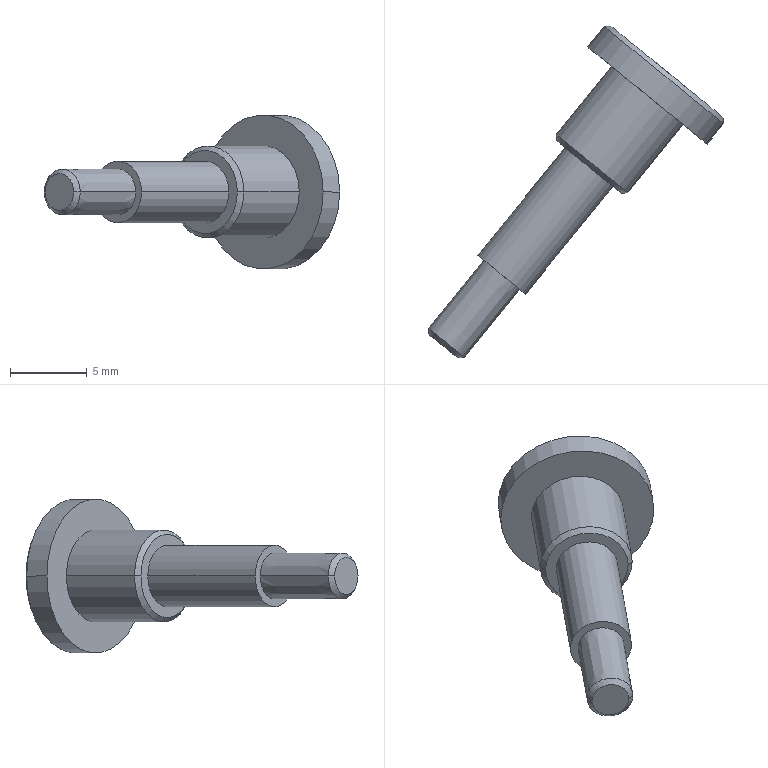Part | SolidWorks | features BaseBody 1 | 1 solid | 23 faces | box 19.175 x 21.566 x 10 mm | volume 474.47 mm3 | cone 8 | cylinder 8 | plane 7 | commonest cylinder face diameters 4 x2 6 x2 10 x2 15 x2
STEP:
#1=CARTESIAN_POINT('',(535.708,-146.474,274.562));
#2=VERTEX_POINT('',#1);
#3=CARTESIAN_POINT('',(543.001,-152.404,274.562));
#4=VERTEX_POINT('',#3);
#5=CARTESIAN_POINT('',(539.354,-149.439,274.562));
#6=DIRECTION('',(0.6309,0.7758,-0.000000012));
#7=DIRECTION('',(0.7758,-0.6309,0.));
#8=AXIS2_PLACEMENT_3D('',#5,#6,#7);
#9=CIRCLE('',#8,4.7);
#10=EDGE_CURVE('',#2,#4,#9,.T.);
#11=ORIENTED_EDGE('',*,*,#10,.F.);
#12=CARTESIAN_POINT('',(535.286,-146.517,274.562));
#13=VERTEX_POINT('',#12);
#14=CARTESIAN_POINT('',(535.286,-146.517,274.562));
#15=DIRECTION('',(-0.9947,-0.1025,0.000000009));
#16=VECTOR('',#15,1000.);
#17=LINE('',#14,#16);
#18=EDGE_CURVE('',#2,#13,#17,.T.);
#19=ORIENTED_EDGE('',*,*,#18,.T.);
#20=CARTESIAN_POINT('',(543.044,-152.826,274.562));
#21=VERTEX_POINT('',#20);
#22=CARTESIAN_POINT('',(539.165,-149.672,274.562));
#23=DIRECTION('',(0.6309,0.7758,-0.000000012));
#24=DIRECTION('',(0.7758,-0.6309,-0.000000063));
#25=AXIS2_PLACEMENT_3D('',#22,#23,#24);
#26=CIRCLE('',#25,5.);
#27=EDGE_CURVE('',#13,#21,#26,.T.);
#28=ORIENTED_EDGE('',*,*,#27,.T.);
#29=CARTESIAN_POINT('',(543.044,-152.826,274.562));
#30=DIRECTION('',(0.1025,-0.9947,0.000000009));
#31=VECTOR('',#30,1000.);
#32=LINE('',#29,#31);
#33=EDGE_CURVE('',#4,#21,#32,.T.);
#34=ORIENTED_EDGE('',*,*,#33,.F.);
#35=EDGE_LOOP('',(#11,#19,#28,#34));
#36=FACE_OUTER_BOUND('',#35,.T.);
#37=CARTESIAN_POINT('',(539.165,-149.672,274.562));
#38=DIRECTION('',(-0.6309,-0.7758,0.000000012));
#39=DIRECTION('',(0.7758,-0.6309,0.));
#40=AXIS2_PLACEMENT_3D('',#37,#38,#39);
#41=CONICAL_SURFACE('',#40,5.,0.7854);
#42=ADVANCED_FACE('',(#36),#41,.T.);
#43=ORIENTED_EDGE('',*,*,#27,.F.);
#44=CARTESIAN_POINT('',(534.213,-147.836,274.562));
#45=VERTEX_POINT('',#44);
#46=CARTESIAN_POINT('',(534.844,-147.06,274.562));
#47=DIRECTION('',(-0.6309,-0.7758,0.000000012));
#48=VECTOR('',#47,1000.);
#49=LINE('',#46,#48);
#50=EDGE_CURVE('',#13,#45,#49,.T.);
#51=ORIENTED_EDGE('',*,*,#50,.T.);
#52=CARTESIAN_POINT('',(541.972,-154.145,274.562));
#53=VERTEX_POINT('',#52);
#54=CARTESIAN_POINT('',(538.092,-150.991,274.562));
#55=DIRECTION('',(0.6309,0.7758,-0.000000012));
#56=DIRECTION('',(0.7758,-0.6309,0.));
#57=AXIS2_PLACEMENT_3D('',#54,#55,#56);
#58=CIRCLE('',#57,5.);
#59=EDGE_CURVE('',#45,#53,#58,.T.);
#60=ORIENTED_EDGE('',*,*,#59,.T.);
#61=CARTESIAN_POINT('',(542.602,-153.37,274.562));
#62=DIRECTION('',(-0.6309,-0.7758,0.000000012));
#63=VECTOR('',#62,1000.);
#64=LINE('',#61,#63);
#65=EDGE_CURVE('',#21,#53,#64,.T.);
#66=ORIENTED_EDGE('',*,*,#65,.F.);
#67=EDGE_LOOP('',(#43,#51,#60,#66));
#68=FACE_OUTER_BOUND('',#67,.T.);
#69=CARTESIAN_POINT('',(538.723,-150.215,274.562));
#70=DIRECTION('',(-0.6309,-0.7758,0.000000012));
#71=DIRECTION('',(0.7758,-0.6309,0.));
#72=AXIS2_PLACEMENT_3D('',#69,#70,#71);
#73=CYLINDRICAL_SURFACE('',#72,5.);
#74=ADVANCED_FACE('',(#68),#73,.T.);
#75=CARTESIAN_POINT('',(539.082,-150.519,274.393));
#76=VERTEX_POINT('',#75);
#77=CARTESIAN_POINT('',(540.707,-150.539,277.93));
#78=VERTEX_POINT('',#77);
#79=CARTESIAN_POINT('',(543.814,-144.701,274.393));
#80=DIRECTION('',(-0.73,0.5937,0.3386));
#81=DIRECTION('',(-0.6309,-0.7758,0.));
#82=AXIS2_PLACEMENT_3D('',#79,#80,#81);
#83=CIRCLE('',#82,7.5);
#84=EDGE_CURVE('',#76,#78,#83,.T.);
#85=ORIENTED_EDGE('',*,*,#84,.F.);
#86=CARTESIAN_POINT('',(538.352,-149.926,274.732));
#87=VERTEX_POINT('',#86);
#88=CARTESIAN_POINT('',(539.082,-150.519,274.393));
#89=DIRECTION('',(-0.73,0.5937,0.3386));
#90=VECTOR('',#89,1000.);
#91=LINE('',#88,#90);
#92=EDGE_CURVE('',#76,#87,#91,.T.);
#93=ORIENTED_EDGE('',*,*,#92,.T.);
#94=CARTESIAN_POINT('',(539.977,-149.945,278.268));
#95=VERTEX_POINT('',#94);
#96=CARTESIAN_POINT('',(543.084,-144.107,274.732));
#97=DIRECTION('',(-0.73,0.5937,0.3386));
#98=DIRECTION('',(-0.6309,-0.7758,0.));
#99=AXIS2_PLACEMENT_3D('',#96,#97,#98);
#100=CIRCLE('',#99,7.5);
#101=EDGE_CURVE('',#87,#95,#100,.T.);
#102=ORIENTED_EDGE('',*,*,#101,.T.);
#103=CARTESIAN_POINT('',(540.707,-150.539,277.93));
#104=DIRECTION('',(-0.73,0.5937,0.3386));
#105=VECTOR('',#104,1000.);
#106=LINE('',#103,#105);
#107=EDGE_CURVE('',#78,#95,#106,.T.);
#108=ORIENTED_EDGE('',*,*,#107,.F.);
#109=EDGE_LOOP('',(#85,#93,#102,#108));
#110=FACE_OUTER_BOUND('',#109,.T.);
#111=CARTESIAN_POINT('',(543.814,-144.701,274.393));
#112=DIRECTION('',(-0.73,0.5937,0.3386));
#113=DIRECTION('',(-0.6309,-0.7758,0.));
#114=AXIS2_PLACEMENT_3D('',#111,#112,#113);
#115=CYLINDRICAL_SURFACE('',#114,7.5);
#116=ADVANCED_FACE('',(#110),#115,.F.);
#117=CARTESIAN_POINT('',(535.765,-149.098,274.562));
#118=VERTEX_POINT('',#117);
#119=CARTESIAN_POINT('',(540.42,-152.884,274.562));
#120=VERTEX_POINT('',#119);
#121=CARTESIAN_POINT('',(538.092,-150.991,274.562));
#122=DIRECTION('',(0.6309,0.7758,-0.000000012));
#123=DIRECTION('',(0.7758,-0.6309,0.));
#124=AXIS2_PLACEMENT_3D('',#121,#122,#123);
#125=CIRCLE('',#124,3.);
#126=EDGE_CURVE('',#118,#120,#125,.T.);
#127=ORIENTED_EDGE('',*,*,#126,.F.);
#128=CARTESIAN_POINT('',(532.169,-153.52,274.562));
#129=VERTEX_POINT('',#128);
#130=CARTESIAN_POINT('',(533.872,-151.425,274.562));
#131=DIRECTION('',(-0.6309,-0.7758,0.000000012));
#132=VECTOR('',#131,1000.);
#133=LINE('',#130,#132);
#134=EDGE_CURVE('',#118,#129,#133,.T.);
#135=ORIENTED_EDGE('',*,*,#134,.T.);
#136=CARTESIAN_POINT('',(536.824,-157.306,274.562));
#137=VERTEX_POINT('',#136);
#138=CARTESIAN_POINT('',(534.496,-155.413,274.562));
#139=DIRECTION('',(0.6309,0.7758,-0.000000012));
#140=DIRECTION('',(0.7758,-0.6309,0.));
#141=AXIS2_PLACEMENT_3D('',#138,#139,#140);
#142=CIRCLE('',#141,3.);
#143=EDGE_CURVE('',#129,#137,#142,.T.);
#144=ORIENTED_EDGE('',*,*,#143,.T.);
#145=CARTESIAN_POINT('',(538.527,-155.211,274.562));
#146=DIRECTION('',(-0.6309,-0.7758,0.000000012));
#147=VECTOR('',#146,1000.);
#148=LINE('',#145,#147);
#149=EDGE_CURVE('',#120,#137,#148,.T.);
#150=ORIENTED_EDGE('',*,*,#149,.F.);
#151=EDGE_LOOP('',(#127,#135,#144,#150));
#152=FACE_OUTER_BOUND('',#151,.T.);
#153=CARTESIAN_POINT('',(536.2,-153.318,274.562));
#154=DIRECTION('',(-0.6309,-0.7758,0.000000012));
#155=DIRECTION('',(0.7758,-0.6309,0.));
#156=AXIS2_PLACEMENT_3D('',#153,#154,#155);
#157=CYLINDRICAL_SURFACE('',#156,3.);
#158=ADVANCED_FACE('',(#152),#157,.T.);
#159=CARTESIAN_POINT('',(532.212,-153.942,274.562));
#160=VERTEX_POINT('',#159);
#161=CARTESIAN_POINT('',(536.402,-157.349,274.562));
#162=VERTEX_POINT('',#161);
#163=CARTESIAN_POINT('',(534.307,-155.646,274.562));
#164=DIRECTION('',(0.6309,0.7758,-0.000000012));
#165=DIRECTION('',(-0.7758,0.6309,0.));
#166=AXIS2_PLACEMENT_3D('',#163,#164,#165);
#167=CIRCLE('',#166,2.7);
#168=EDGE_CURVE('',#160,#162,#167,.T.);
#169=ORIENTED_EDGE('',*,*,#168,.T.);
#170=CARTESIAN_POINT('',(536.824,-157.306,274.562));
#171=DIRECTION('',(0.9947,0.1025,-0.000000009));
#172=VECTOR('',#171,1000.);
#173=LINE('',#170,#172);
#174=EDGE_CURVE('',#162,#137,#173,.T.);
#175=ORIENTED_EDGE('',*,*,#174,.T.);
#176=ORIENTED_EDGE('',*,*,#143,.F.);
#177=CARTESIAN_POINT('',(532.169,-153.52,274.562));
#178=DIRECTION('',(-0.1025,0.9947,-0.000000009));
#179=VECTOR('',#178,1000.);
#180=LINE('',#177,#179);
#181=EDGE_CURVE('',#160,#129,#180,.T.);
#182=ORIENTED_EDGE('',*,*,#181,.F.);
#183=EDGE_LOOP('',(#169,#175,#176,#182));
#184=FACE_OUTER_BOUND('',#183,.T.);
#185=CARTESIAN_POINT('',(534.496,-155.413,274.562));
#186=DIRECTION('',(0.6309,0.7758,-0.000000012));
#187=DIRECTION('',(-0.7758,0.6309,0.));
#188=AXIS2_PLACEMENT_3D('',#185,#186,#187);
#189=CONICAL_SURFACE('',#188,3.,0.7854);
#190=ADVANCED_FACE('',(#184),#189,.T.);
#191=CARTESIAN_POINT('',(532.755,-154.384,274.562));
#192=VERTEX_POINT('',#191);
#193=CARTESIAN_POINT('',(535.858,-156.908,274.562));
#194=VERTEX_POINT('',#193);
#195=CARTESIAN_POINT('',(534.307,-155.646,274.562));
#196=DIRECTION('',(0.6309,0.7758,-0.000000012));
#197=DIRECTION('',(0.7758,-0.6309,0.));
#198=AXIS2_PLACEMENT_3D('',#195,#196,#197);
#199=CIRCLE('',#198,2.);
#200=EDGE_CURVE('',#192,#194,#199,.T.);
#201=ORIENTED_EDGE('',*,*,#200,.F.);
#202=CARTESIAN_POINT('',(527.077,-161.366,274.562));
#203=VERTEX_POINT('',#202);
#204=CARTESIAN_POINT('',(529.916,-157.875,274.562));
#205=DIRECTION('',(-0.6309,-0.7758,0.000000012));
#206=VECTOR('',#205,1000.);
#207=LINE('',#204,#206);
#208=EDGE_CURVE('',#192,#203,#207,.T.);
#209=ORIENTED_EDGE('',*,*,#208,.T.);
#210=CARTESIAN_POINT('',(530.18,-163.89,274.562));
#211=VERTEX_POINT('',#210);
#212=CARTESIAN_POINT('',(528.628,-162.628,274.562));
#213=DIRECTION('',(0.6309,0.7758,-0.000000012));
#214=DIRECTION('',(0.7758,-0.6309,0.));
#215=AXIS2_PLACEMENT_3D('',#212,#213,#214);
#216=CIRCLE('',#215,2.);
#217=EDGE_CURVE('',#203,#211,#216,.T.);
#218=ORIENTED_EDGE('',*,*,#217,.T.);
#219=CARTESIAN_POINT('',(533.019,-160.399,274.562));
#220=DIRECTION('',(-0.6309,-0.7758,0.000000012));
#221=VECTOR('',#220,1000.);
#222=LINE('',#219,#221);
#223=EDGE_CURVE('',#194,#211,#222,.T.);
#224=ORIENTED_EDGE('',*,*,#223,.F.);
#225=EDGE_LOOP('',(#201,#209,#218,#224));
#226=FACE_OUTER_BOUND('',#225,.T.);
#227=CARTESIAN_POINT('',(531.468,-159.137,274.562));
#228=DIRECTION('',(-0.6309,-0.7758,0.000000012));
#229=DIRECTION('',(0.7758,-0.6309,0.));
#230=AXIS2_PLACEMENT_3D('',#227,#228,#229);
#231=CYLINDRICAL_SURFACE('',#230,2.);
#232=ADVANCED_FACE('',(#226),#231,.T.);
#233=CARTESIAN_POINT('',(523.869,-166.105,274.562));
#234=VERTEX_POINT('',#233);
#235=CARTESIAN_POINT('',(526.195,-167.996,274.562));
#236=VERTEX_POINT('',#235);
#237=CARTESIAN_POINT('',(525.032,-167.051,274.562));
#238=DIRECTION('',(0.6309,0.7758,-0.000000012));
#239=DIRECTION('',(-0.7758,0.6309,0.000000063));
#240=AXIS2_PLACEMENT_3D('',#237,#238,#239);
#241=CIRCLE('',#240,1.499);
#242=EDGE_CURVE('',#234,#236,#241,.T.);
#243=ORIENTED_EDGE('',*,*,#242,.T.);
#244=CARTESIAN_POINT('',(529.792,-163.575,274.562));
#245=VERTEX_POINT('',#244);
#246=CARTESIAN_POINT('',(529.792,-163.575,274.562));
#247=DIRECTION('',(0.6311,0.7757,-0.000000012));
#248=VECTOR('',#247,1000.);
#249=LINE('',#246,#248);
#250=EDGE_CURVE('',#236,#245,#249,.T.);
#251=ORIENTED_EDGE('',*,*,#250,.T.);
#252=CARTESIAN_POINT('',(527.465,-161.682,274.562));
#253=VERTEX_POINT('',#252);
#254=CARTESIAN_POINT('',(528.628,-162.628,274.562));
#255=DIRECTION('',(0.6309,0.7758,-0.000000012));
#256=DIRECTION('',(-0.7758,0.6309,0.));
#257=AXIS2_PLACEMENT_3D('',#254,#255,#256);
#258=CIRCLE('',#257,1.5);
#259=EDGE_CURVE('',#253,#245,#258,.T.);
#260=ORIENTED_EDGE('',*,*,#259,.F.);
#261=CARTESIAN_POINT('',(527.465,-161.682,274.562));
#262=DIRECTION('',(0.6308,0.7759,-0.000000012));
#263=VECTOR('',#262,1000.);
#264=LINE('',#261,#263);
#265=EDGE_CURVE('',#234,#253,#264,.T.);
#266=ORIENTED_EDGE('',*,*,#265,.F.);
#267=EDGE_LOOP('',(#243,#251,#260,#266));
#268=FACE_OUTER_BOUND('',#267,.T.);
#269=CARTESIAN_POINT('',(528.628,-162.628,274.562));
#270=DIRECTION('',(0.6309,0.7758,-0.000000012));
#271=DIRECTION('',(-0.7758,0.6309,0.));
#272=AXIS2_PLACEMENT_3D('',#269,#270,#271);
#273=CONICAL_SURFACE('',#272,1.5,0.0001745);
#274=ADVANCED_FACE('',(#268),#273,.T.);
#275=CARTESIAN_POINT('',(523.913,-166.527,274.562));
#276=VERTEX_POINT('',#275);
#277=CARTESIAN_POINT('',(525.773,-168.04,274.562));
#278=VERTEX_POINT('',#277);
#279=CARTESIAN_POINT('',(524.843,-167.283,274.562));
#280=DIRECTION('',(0.6309,0.7758,-0.000000012));
#281=DIRECTION('',(-0.7758,0.6309,0.));
#282=AXIS2_PLACEMENT_3D('',#279,#280,#281);
#283=CIRCLE('',#282,1.199);
#284=EDGE_CURVE('',#276,#278,#283,.T.);
#285=ORIENTED_EDGE('',*,*,#284,.T.);
#286=CARTESIAN_POINT('',(526.195,-167.996,274.562));
#287=DIRECTION('',(0.9947,0.1024,-0.000000009));
#288=VECTOR('',#287,1000.);
#289=LINE('',#286,#288);
#290=EDGE_CURVE('',#278,#236,#289,.T.);
#291=ORIENTED_EDGE('',*,*,#290,.T.);
#292=ORIENTED_EDGE('',*,*,#242,.F.);
#293=CARTESIAN_POINT('',(523.869,-166.105,274.562));
#294=DIRECTION('',(-0.1026,0.9947,-0.000000009));
#295=VECTOR('',#294,1000.);
#296=LINE('',#293,#295);
#297=EDGE_CURVE('',#276,#234,#296,.T.);
#298=ORIENTED_EDGE('',*,*,#297,.F.);
#299=EDGE_LOOP('',(#285,#291,#292,#298));
#300=FACE_OUTER_BOUND('',#299,.T.);
#301=CARTESIAN_POINT('',(525.032,-167.051,274.562));
#302=DIRECTION('',(0.6309,0.7758,-0.000000012));
#303=DIRECTION('',(-0.7758,0.6309,0.));
#304=AXIS2_PLACEMENT_3D('',#301,#302,#303);
#305=CONICAL_SURFACE('',#304,1.499,0.7855);
#306=ADVANCED_FACE('',(#300),#305,.T.);
#307=CARTESIAN_POINT('',(539.354,-149.439,274.562));
#308=DIRECTION('',(0.6309,0.7758,-0.000000012));
#309=DIRECTION('',(0.7758,-0.6309,0.));
#310=AXIS2_PLACEMENT_3D('',#307,#308,#309);
#311=CIRCLE('',#310,4.7);
#312=EDGE_CURVE('',#4,#2,#311,.T.);
#313=ORIENTED_EDGE('',*,*,#312,.T.);
#314=ORIENTED_EDGE('',*,*,#10,.T.);
#315=EDGE_LOOP('',(#313,#314));
#316=FACE_OUTER_BOUND('',#315,.T.);
#317=ORIENTED_EDGE('',*,*,#107,.T.);
#318=CARTESIAN_POINT('',(538.002,-148.339,271.195));
#319=VERTEX_POINT('',#318);
#320=CARTESIAN_POINT('',(539.977,-149.945,278.268));
#321=DIRECTION('',(-0.2627,0.2136,-0.9409));
#322=VECTOR('',#321,1000.);
#323=LINE('',#320,#322);
#324=EDGE_CURVE('',#95,#319,#323,.T.);
#325=ORIENTED_EDGE('',*,*,#324,.T.);
#326=CARTESIAN_POINT('',(538.732,-148.933,270.856));
#327=VERTEX_POINT('',#326);
#328=CARTESIAN_POINT('',(538.732,-148.933,270.856));
#329=DIRECTION('',(0.73,-0.5937,-0.3386));
#330=VECTOR('',#329,1000.);
#331=LINE('',#328,#330);
#332=EDGE_CURVE('',#319,#327,#331,.T.);
#333=ORIENTED_EDGE('',*,*,#332,.T.);
#334=CARTESIAN_POINT('',(538.732,-148.933,270.856));
#335=DIRECTION('',(0.2627,-0.2136,0.9409));
#336=VECTOR('',#335,1000.);
#337=LINE('',#334,#336);
#338=EDGE_CURVE('',#327,#78,#337,.T.);
#339=ORIENTED_EDGE('',*,*,#338,.T.);
#340=EDGE_LOOP('',(#317,#325,#333,#339));
#341=FACE_BOUND('',#340,.T.);
#342=CARTESIAN_POINT('',(537.415,-147.862,274.562));
#343=DIRECTION('',(0.6309,0.7758,-0.000000012));
#344=DIRECTION('',(-0.7758,0.6309,0.));
#345=AXIS2_PLACEMENT_3D('',#342,#343,#344);
#346=PLANE('',#345);
#347=ADVANCED_FACE('',(#316,#341),#346,.T.);
#348=ORIENTED_EDGE('',*,*,#18,.F.);
#349=ORIENTED_EDGE('',*,*,#312,.F.);
#350=ORIENTED_EDGE('',*,*,#33,.T.);
#351=CARTESIAN_POINT('',(539.165,-149.672,274.562));
#352=DIRECTION('',(0.6309,0.7758,-0.000000012));
#353=DIRECTION('',(0.7758,-0.6309,-0.000000063));
#354=AXIS2_PLACEMENT_3D('',#351,#352,#353);
#355=CIRCLE('',#354,5.);
#356=EDGE_CURVE('',#21,#13,#355,.T.);
#357=ORIENTED_EDGE('',*,*,#356,.T.);
#358=EDGE_LOOP('',(#348,#349,#350,#357));
#359=FACE_OUTER_BOUND('',#358,.T.);
#360=CARTESIAN_POINT('',(539.165,-149.672,274.562));
#361=DIRECTION('',(-0.6309,-0.7758,0.000000012));
#362=DIRECTION('',(0.7758,-0.6309,0.));
#363=AXIS2_PLACEMENT_3D('',#360,#361,#362);
#364=CONICAL_SURFACE('',#363,5.,0.7854);
#365=ADVANCED_FACE('',(#359),#364,.T.);
#366=CARTESIAN_POINT('',(543.084,-144.107,274.732));
#367=DIRECTION('',(-0.73,0.5937,0.3386));
#368=DIRECTION('',(-0.6309,-0.7758,0.));
#369=AXIS2_PLACEMENT_3D('',#366,#367,#368);
#370=CIRCLE('',#369,7.5);
#371=EDGE_CURVE('',#319,#87,#370,.T.);
#372=ORIENTED_EDGE('',*,*,#371,.F.);
#373=ORIENTED_EDGE('',*,*,#324,.F.);
#374=ORIENTED_EDGE('',*,*,#101,.F.);
#375=EDGE_LOOP('',(#372,#373,#374));
#376=FACE_OUTER_BOUND('',#375,.T.);
#377=CARTESIAN_POINT('',(543.084,-144.107,274.732));
#378=DIRECTION('',(-0.73,0.5937,0.3386));
#379=DIRECTION('',(-0.6309,-0.7758,0.));
#380=AXIS2_PLACEMENT_3D('',#377,#378,#379);
#381=PLANE('',#380);
#382=ADVANCED_FACE('',(#376),#381,.F.);
#383=ORIENTED_EDGE('',*,*,#338,.F.);
#384=CARTESIAN_POINT('',(543.814,-144.701,274.393));
#385=DIRECTION('',(-0.73,0.5937,0.3386));
#386=DIRECTION('',(-0.6309,-0.7758,0.));
#387=AXIS2_PLACEMENT_3D('',#384,#385,#386);
#388=CIRCLE('',#387,7.5);
#389=EDGE_CURVE('',#327,#76,#388,.T.);
#390=ORIENTED_EDGE('',*,*,#389,.T.);
#391=ORIENTED_EDGE('',*,*,#84,.T.);
#392=EDGE_LOOP('',(#383,#390,#391));
#393=FACE_OUTER_BOUND('',#392,.T.);
#394=CARTESIAN_POINT('',(543.814,-144.701,274.393));
#395=DIRECTION('',(-0.73,0.5937,0.3386));
#396=DIRECTION('',(-0.6309,-0.7758,0.));
#397=AXIS2_PLACEMENT_3D('',#394,#395,#396);
#398=PLANE('',#397);
#399=ADVANCED_FACE('',(#393),#398,.T.);
#400=ORIENTED_EDGE('',*,*,#50,.F.);
#401=ORIENTED_EDGE('',*,*,#356,.F.);
#402=ORIENTED_EDGE('',*,*,#65,.T.);
#403=CARTESIAN_POINT('',(538.092,-150.991,274.562));
#404=DIRECTION('',(0.6309,0.7758,-0.000000012));
#405=DIRECTION('',(0.7758,-0.6309,0.));
#406=AXIS2_PLACEMENT_3D('',#403,#404,#405);
#407=CIRCLE('',#406,5.);
#408=EDGE_CURVE('',#53,#45,#407,.T.);
#409=ORIENTED_EDGE('',*,*,#408,.T.);
#410=EDGE_LOOP('',(#400,#401,#402,#409));
#411=FACE_OUTER_BOUND('',#410,.T.);
#412=CARTESIAN_POINT('',(538.723,-150.215,274.562));
#413=DIRECTION('',(-0.6309,-0.7758,0.000000012));
#414=DIRECTION('',(0.7758,-0.6309,0.));
#415=AXIS2_PLACEMENT_3D('',#412,#413,#414);
#416=CYLINDRICAL_SURFACE('',#415,5.);
#417=ADVANCED_FACE('',(#411),#416,.T.);
#418=ORIENTED_EDGE('',*,*,#92,.F.);
#419=ORIENTED_EDGE('',*,*,#389,.F.);
#420=ORIENTED_EDGE('',*,*,#332,.F.);
#421=ORIENTED_EDGE('',*,*,#371,.T.);
#422=EDGE_LOOP('',(#418,#419,#420,#421));
#423=FACE_OUTER_BOUND('',#422,.T.);
#424=CARTESIAN_POINT('',(543.814,-144.701,274.393));
#425=DIRECTION('',(-0.73,0.5937,0.3386));
#426=DIRECTION('',(-0.6309,-0.7758,0.));
#427=AXIS2_PLACEMENT_3D('',#424,#425,#426);
#428=CYLINDRICAL_SURFACE('',#427,7.5);
#429=ADVANCED_FACE('',(#423),#428,.F.);
#430=CARTESIAN_POINT('',(538.092,-150.991,274.562));
#431=DIRECTION('',(0.6309,0.7758,-0.000000012));
#432=DIRECTION('',(0.7758,-0.6309,0.));
#433=AXIS2_PLACEMENT_3D('',#430,#431,#432);
#434=CIRCLE('',#433,3.);
#435=EDGE_CURVE('',#120,#118,#434,.T.);
#436=ORIENTED_EDGE('',*,*,#435,.T.);
#437=ORIENTED_EDGE('',*,*,#126,.T.);
#438=EDGE_LOOP('',(#436,#437));
#439=FACE_BOUND('',#438,.T.);
#440=ORIENTED_EDGE('',*,*,#408,.F.);
#441=ORIENTED_EDGE('',*,*,#59,.F.);
#442=EDGE_LOOP('',(#440,#441));
#443=FACE_OUTER_BOUND('',#442,.T.);
#444=CARTESIAN_POINT('',(534.989,-148.467,274.562));
#445=DIRECTION('',(-0.6309,-0.7758,0.000000012));
#446=DIRECTION('',(0.7758,-0.6309,0.));
#447=AXIS2_PLACEMENT_3D('',#444,#445,#446);
#448=PLANE('',#447);
#449=ADVANCED_FACE('',(#439,#443),#448,.T.);
#450=ORIENTED_EDGE('',*,*,#134,.F.);
#451=ORIENTED_EDGE('',*,*,#435,.F.);
#452=ORIENTED_EDGE('',*,*,#149,.T.);
#453=CARTESIAN_POINT('',(534.496,-155.413,274.562));
#454=DIRECTION('',(0.6309,0.7758,-0.000000012));
#455=DIRECTION('',(0.7758,-0.6309,0.));
#456=AXIS2_PLACEMENT_3D('',#453,#454,#455);
#457=CIRCLE('',#456,3.);
#458=EDGE_CURVE('',#137,#129,#457,.T.);
#459=ORIENTED_EDGE('',*,*,#458,.T.);
#460=EDGE_LOOP('',(#450,#451,#452,#459));
#461=FACE_OUTER_BOUND('',#460,.T.);
#462=CARTESIAN_POINT('',(536.2,-153.318,274.562));
#463=DIRECTION('',(-0.6309,-0.7758,0.000000012));
#464=DIRECTION('',(0.7758,-0.6309,0.));
#465=AXIS2_PLACEMENT_3D('',#462,#463,#464);
#466=CYLINDRICAL_SURFACE('',#465,3.);
#467=ADVANCED_FACE('',(#461),#466,.T.);
#468=ORIENTED_EDGE('',*,*,#174,.F.);
#469=CARTESIAN_POINT('',(534.307,-155.646,274.562));
#470=DIRECTION('',(0.6309,0.7758,-0.000000012));
#471=DIRECTION('',(-0.7758,0.6309,0.));
#472=AXIS2_PLACEMENT_3D('',#469,#470,#471);
#473=CIRCLE('',#472,2.7);
#474=EDGE_CURVE('',#162,#160,#473,.T.);
#475=ORIENTED_EDGE('',*,*,#474,.T.);
#476=ORIENTED_EDGE('',*,*,#181,.T.);
#477=ORIENTED_EDGE('',*,*,#458,.F.);
#478=EDGE_LOOP('',(#468,#475,#476,#477));
#479=FACE_OUTER_BOUND('',#478,.T.);
#480=CARTESIAN_POINT('',(534.496,-155.413,274.562));
#481=DIRECTION('',(0.6309,0.7758,-0.000000012));
#482=DIRECTION('',(-0.7758,0.6309,0.));
#483=AXIS2_PLACEMENT_3D('',#480,#481,#482);
#484=CONICAL_SURFACE('',#483,3.,0.7854);
#485=ADVANCED_FACE('',(#479),#484,.T.);
#486=ORIENTED_EDGE('',*,*,#168,.F.);
#487=ORIENTED_EDGE('',*,*,#474,.F.);
#488=EDGE_LOOP('',(#486,#487));
#489=FACE_OUTER_BOUND('',#488,.T.);
#490=CARTESIAN_POINT('',(534.307,-155.646,274.562));
#491=DIRECTION('',(0.6309,0.7758,-0.000000012));
#492=DIRECTION('',(0.7758,-0.6309,0.));
#493=AXIS2_PLACEMENT_3D('',#490,#491,#492);
#494=CIRCLE('',#493,2.);
#495=EDGE_CURVE('',#194,#192,#494,.T.);
#496=ORIENTED_EDGE('',*,*,#495,.T.);
#497=ORIENTED_EDGE('',*,*,#200,.T.);
#498=EDGE_LOOP('',(#496,#497));
#499=FACE_BOUND('',#498,.T.);
#500=CARTESIAN_POINT('',(532.367,-154.068,274.562));
#501=DIRECTION('',(-0.6309,-0.7758,0.000000012));
#502=DIRECTION('',(0.7758,-0.6309,0.));
#503=AXIS2_PLACEMENT_3D('',#500,#501,#502);
#504=PLANE('',#503);
#505=ADVANCED_FACE('',(#489,#499),#504,.T.);
#506=ORIENTED_EDGE('',*,*,#208,.F.);
#507=ORIENTED_EDGE('',*,*,#495,.F.);
#508=ORIENTED_EDGE('',*,*,#223,.T.);
#509=CARTESIAN_POINT('',(528.628,-162.628,274.562));
#510=DIRECTION('',(0.6309,0.7758,-0.000000012));
#511=DIRECTION('',(0.7758,-0.6309,0.));
#512=AXIS2_PLACEMENT_3D('',#509,#510,#511);
#513=CIRCLE('',#512,2.);
#514=EDGE_CURVE('',#211,#203,#513,.T.);
#515=ORIENTED_EDGE('',*,*,#514,.T.);
#516=EDGE_LOOP('',(#506,#507,#508,#515));
#517=FACE_OUTER_BOUND('',#516,.T.);
#518=CARTESIAN_POINT('',(531.468,-159.137,274.562));
#519=DIRECTION('',(-0.6309,-0.7758,0.000000012));
#520=DIRECTION('',(0.7758,-0.6309,0.));
#521=AXIS2_PLACEMENT_3D('',#518,#519,#520);
#522=CYLINDRICAL_SURFACE('',#521,2.);
#523=ADVANCED_FACE('',(#517),#522,.T.);
#524=ORIENTED_EDGE('',*,*,#514,.F.);
#525=ORIENTED_EDGE('',*,*,#217,.F.);
#526=EDGE_LOOP('',(#524,#525));
#527=FACE_OUTER_BOUND('',#526,.T.);
#528=ORIENTED_EDGE('',*,*,#259,.T.);
#529=CARTESIAN_POINT('',(528.628,-162.628,274.562));
#530=DIRECTION('',(0.6309,0.7758,-0.000000012));
#531=DIRECTION('',(-0.7758,0.6309,0.));
#532=AXIS2_PLACEMENT_3D('',#529,#530,#531);
#533=CIRCLE('',#532,1.5);
#534=EDGE_CURVE('',#245,#253,#533,.T.);
#535=ORIENTED_EDGE('',*,*,#534,.T.);
#536=EDGE_LOOP('',(#528,#535));
#537=FACE_BOUND('',#536,.T.);
#538=CARTESIAN_POINT('',(527.853,-161.997,274.562));
#539=DIRECTION('',(-0.6309,-0.7758,0.000000012));
#540=DIRECTION('',(0.7758,-0.6309,0.));
#541=AXIS2_PLACEMENT_3D('',#538,#539,#540);
#542=PLANE('',#541);
#543=ADVANCED_FACE('',(#527,#537),#542,.T.);
#544=ORIENTED_EDGE('',*,*,#250,.F.);
#545=CARTESIAN_POINT('',(525.032,-167.051,274.562));
#546=DIRECTION('',(0.6309,0.7758,-0.000000012));
#547=DIRECTION('',(-0.7758,0.6309,0.000000063));
#548=AXIS2_PLACEMENT_3D('',#545,#546,#547);
#549=CIRCLE('',#548,1.499);
#550=EDGE_CURVE('',#236,#234,#549,.T.);
#551=ORIENTED_EDGE('',*,*,#550,.T.);
#552=ORIENTED_EDGE('',*,*,#265,.T.);
#553=ORIENTED_EDGE('',*,*,#534,.F.);
#554=EDGE_LOOP('',(#544,#551,#552,#553));
#555=FACE_OUTER_BOUND('',#554,.T.);
#556=CARTESIAN_POINT('',(528.628,-162.628,274.562));
#557=DIRECTION('',(0.6309,0.7758,-0.000000012));
#558=DIRECTION('',(-0.7758,0.6309,0.));
#559=AXIS2_PLACEMENT_3D('',#556,#557,#558);
#560=CONICAL_SURFACE('',#559,1.5,0.0001745);
#561=ADVANCED_FACE('',(#555),#560,.T.);
#562=ORIENTED_EDGE('',*,*,#290,.F.);
#563=CARTESIAN_POINT('',(524.843,-167.283,274.562));
#564=DIRECTION('',(0.6309,0.7758,-0.000000012));
#565=DIRECTION('',(-0.7758,0.6309,0.));
#566=AXIS2_PLACEMENT_3D('',#563,#564,#565);
#567=CIRCLE('',#566,1.199);
#568=EDGE_CURVE('',#278,#276,#567,.T.);
#569=ORIENTED_EDGE('',*,*,#568,.T.);
#570=ORIENTED_EDGE('',*,*,#297,.T.);
#571=ORIENTED_EDGE('',*,*,#550,.F.);
#572=EDGE_LOOP('',(#562,#569,#570,#571));
#573=FACE_OUTER_BOUND('',#572,.T.);
#574=CARTESIAN_POINT('',(525.032,-167.051,274.562));
#575=DIRECTION('',(0.6309,0.7758,-0.000000012));
#576=DIRECTION('',(-0.7758,0.6309,0.));
#577=AXIS2_PLACEMENT_3D('',#574,#575,#576);
#578=CONICAL_SURFACE('',#577,1.499,0.7855);
#579=ADVANCED_FACE('',(#573),#578,.T.);
#580=ORIENTED_EDGE('',*,*,#284,.F.);
#581=ORIENTED_EDGE('',*,*,#568,.F.);
#582=EDGE_LOOP('',(#580,#581));
#583=FACE_OUTER_BOUND('',#582,.T.);
#584=CARTESIAN_POINT('',(524.843,-167.283,274.562));
#585=DIRECTION('',(-0.6309,-0.7758,0.000000012));
#586=DIRECTION('',(0.7758,-0.6309,0.));
#587=AXIS2_PLACEMENT_3D('',#584,#585,#586);
#588=PLANE('',#587);
#589=ADVANCED_FACE('',(#583),#588,.T.);
#590=CLOSED_SHELL('',(#42,#74,#116,#158,#190,#232,#274,#306,#347,#365,#382,#399,#417,#429,#449,#467,#485,#505,#523,#543,#561,#579,#589));
#591=MANIFOLD_SOLID_BREP('',#590);
#592=CARTESIAN_POINT('',(0.,0.,0.));
#593=DIRECTION('',(0.,0.,1.));
#594=DIRECTION('',(1.,0.,0.));
#595=AXIS2_PLACEMENT_3D('',#592,#593,#594);
#596=(LENGTH_UNIT()NAMED_UNIT(*)SI_UNIT(.MILLI.,.METRE.));
#597=UNCERTAINTY_MEASURE_WITH_UNIT(LENGTH_MEASURE(0.00001),#596,'','');
#598=(NAMED_UNIT(*)PLANE_ANGLE_UNIT()SI_UNIT($,.RADIAN.));
#599=(NAMED_UNIT(*)SI_UNIT($,.STERADIAN.)SOLID_ANGLE_UNIT());
#600=(GEOMETRIC_REPRESENTATION_CONTEXT(3)GLOBAL_UNCERTAINTY_ASSIGNED_CONTEXT((#597))GLOBAL_UNIT_ASSIGNED_CONTEXT((#596,#598,#599))REPRESENTATION_CONTEXT('',''));
#601=ADVANCED_BREP_SHAPE_REPRESENTATION('',(#591,#595),#600);